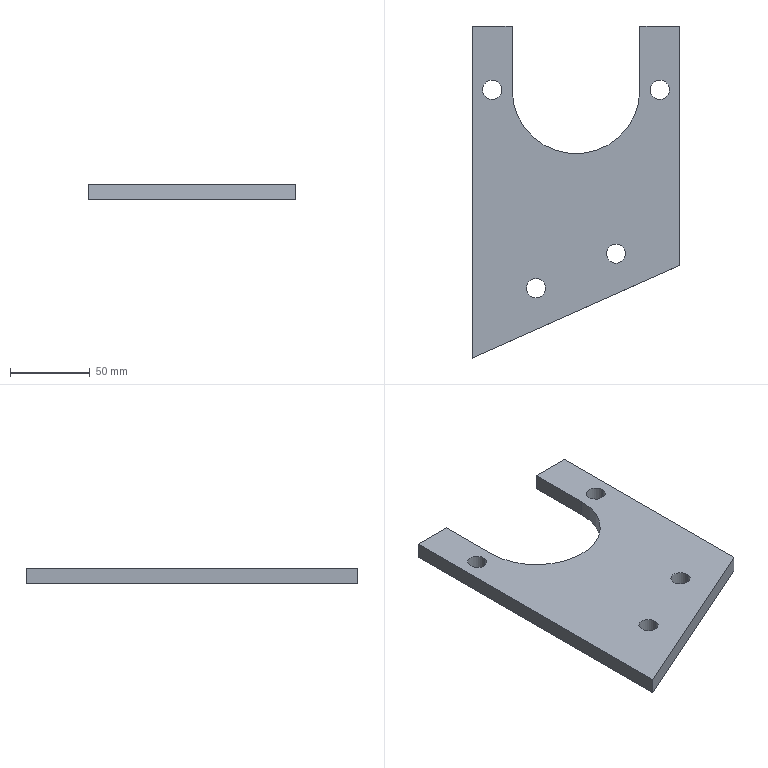Part | SolidWorks | features Extrusion 1 | 1 solid | 18 faces | box 130 x 208 x 10 mm | volume 171043 mm3 | cylinder 9 | plane 9 | commonest cylinder face diameters 12 x8 80 x1
STEP:
#1=CARTESIAN_POINT('',(84.,65.43,10.));
#2=VERTEX_POINT('',#1);
#3=CARTESIAN_POINT('',(96.,65.43,10.));
#4=VERTEX_POINT('',#3);
#5=CARTESIAN_POINT('',(90.,65.43,10.));
#6=DIRECTION('',(0.,0.,1.));
#7=DIRECTION('',(1.,0.,0.));
#8=AXIS2_PLACEMENT_3D('',#5,#6,#7);
#9=CIRCLE('',#8,6.);
#10=EDGE_CURVE('',#2,#4,#9,.T.);
#11=ORIENTED_EDGE('',*,*,#10,.T.);
#12=CARTESIAN_POINT('',(96.,65.43,0.));
#13=VERTEX_POINT('',#12);
#14=CARTESIAN_POINT('',(96.,65.43,10.));
#15=DIRECTION('',(0.,0.,-1.));
#16=VECTOR('',#15,1000.);
#17=LINE('',#14,#16);
#18=EDGE_CURVE('',#4,#13,#17,.T.);
#19=ORIENTED_EDGE('',*,*,#18,.T.);
#20=CARTESIAN_POINT('',(84.,65.43,0.));
#21=VERTEX_POINT('',#20);
#22=CARTESIAN_POINT('',(90.,65.43,0.));
#23=DIRECTION('',(0.,0.,1.));
#24=DIRECTION('',(1.,0.,0.));
#25=AXIS2_PLACEMENT_3D('',#22,#23,#24);
#26=CIRCLE('',#25,6.);
#27=EDGE_CURVE('',#21,#13,#26,.T.);
#28=ORIENTED_EDGE('',*,*,#27,.F.);
#29=CARTESIAN_POINT('',(84.,65.43,10.));
#30=DIRECTION('',(0.,0.,-1.));
#31=VECTOR('',#30,1000.);
#32=LINE('',#29,#31);
#33=EDGE_CURVE('',#2,#21,#32,.T.);
#34=ORIENTED_EDGE('',*,*,#33,.F.);
#35=EDGE_LOOP('',(#11,#19,#28,#34));
#36=FACE_OUTER_BOUND('',#35,.T.);
#37=CARTESIAN_POINT('',(90.,65.43,10.));
#38=DIRECTION('',(0.,0.,-1.));
#39=DIRECTION('',(-1.,0.,0.));
#40=AXIS2_PLACEMENT_3D('',#37,#38,#39);
#41=CYLINDRICAL_SURFACE('',#40,6.);
#42=ADVANCED_FACE('',(#36),#41,.F.);
#43=CARTESIAN_POINT('',(34.,43.72,10.));
#44=VERTEX_POINT('',#43);
#45=CARTESIAN_POINT('',(46.,43.72,10.));
#46=VERTEX_POINT('',#45);
#47=CARTESIAN_POINT('',(40.,43.72,10.));
#48=DIRECTION('',(0.,0.,1.));
#49=DIRECTION('',(1.,0.,0.));
#50=AXIS2_PLACEMENT_3D('',#47,#48,#49);
#51=CIRCLE('',#50,6.);
#52=EDGE_CURVE('',#44,#46,#51,.T.);
#53=ORIENTED_EDGE('',*,*,#52,.T.);
#54=CARTESIAN_POINT('',(46.,43.72,0.));
#55=VERTEX_POINT('',#54);
#56=CARTESIAN_POINT('',(46.,43.72,10.));
#57=DIRECTION('',(0.,0.,-1.));
#58=VECTOR('',#57,1000.);
#59=LINE('',#56,#58);
#60=EDGE_CURVE('',#46,#55,#59,.T.);
#61=ORIENTED_EDGE('',*,*,#60,.T.);
#62=CARTESIAN_POINT('',(34.,43.72,0.));
#63=VERTEX_POINT('',#62);
#64=CARTESIAN_POINT('',(40.,43.72,0.));
#65=DIRECTION('',(0.,0.,1.));
#66=DIRECTION('',(1.,0.,0.));
#67=AXIS2_PLACEMENT_3D('',#64,#65,#66);
#68=CIRCLE('',#67,6.);
#69=EDGE_CURVE('',#63,#55,#68,.T.);
#70=ORIENTED_EDGE('',*,*,#69,.F.);
#71=CARTESIAN_POINT('',(34.,43.72,10.));
#72=DIRECTION('',(0.,0.,-1.));
#73=VECTOR('',#72,1000.);
#74=LINE('',#71,#73);
#75=EDGE_CURVE('',#44,#63,#74,.T.);
#76=ORIENTED_EDGE('',*,*,#75,.F.);
#77=EDGE_LOOP('',(#53,#61,#70,#76));
#78=FACE_OUTER_BOUND('',#77,.T.);
#79=CARTESIAN_POINT('',(40.,43.72,10.));
#80=DIRECTION('',(0.,0.,-1.));
#81=DIRECTION('',(-1.,0.,0.));
#82=AXIS2_PLACEMENT_3D('',#79,#80,#81);
#83=CYLINDRICAL_SURFACE('',#82,6.);
#84=ADVANCED_FACE('',(#78),#83,.F.);
#85=CARTESIAN_POINT('',(6.5,168.,10.));
#86=VERTEX_POINT('',#85);
#87=CARTESIAN_POINT('',(18.5,168.,10.));
#88=VERTEX_POINT('',#87);
#89=CARTESIAN_POINT('',(12.5,168.,10.));
#90=DIRECTION('',(0.,0.,1.));
#91=DIRECTION('',(1.,0.,0.));
#92=AXIS2_PLACEMENT_3D('',#89,#90,#91);
#93=CIRCLE('',#92,6.);
#94=EDGE_CURVE('',#86,#88,#93,.T.);
#95=ORIENTED_EDGE('',*,*,#94,.T.);
#96=CARTESIAN_POINT('',(18.5,168.,0.));
#97=VERTEX_POINT('',#96);
#98=CARTESIAN_POINT('',(18.5,168.,10.));
#99=DIRECTION('',(0.,0.,-1.));
#100=VECTOR('',#99,1000.);
#101=LINE('',#98,#100);
#102=EDGE_CURVE('',#88,#97,#101,.T.);
#103=ORIENTED_EDGE('',*,*,#102,.T.);
#104=CARTESIAN_POINT('',(6.5,168.,0.));
#105=VERTEX_POINT('',#104);
#106=CARTESIAN_POINT('',(12.5,168.,0.));
#107=DIRECTION('',(0.,0.,1.));
#108=DIRECTION('',(1.,0.,0.));
#109=AXIS2_PLACEMENT_3D('',#106,#107,#108);
#110=CIRCLE('',#109,6.);
#111=EDGE_CURVE('',#105,#97,#110,.T.);
#112=ORIENTED_EDGE('',*,*,#111,.F.);
#113=CARTESIAN_POINT('',(6.5,168.,10.));
#114=DIRECTION('',(0.,0.,-1.));
#115=VECTOR('',#114,1000.);
#116=LINE('',#113,#115);
#117=EDGE_CURVE('',#86,#105,#116,.T.);
#118=ORIENTED_EDGE('',*,*,#117,.F.);
#119=EDGE_LOOP('',(#95,#103,#112,#118));
#120=FACE_OUTER_BOUND('',#119,.T.);
#121=CARTESIAN_POINT('',(12.5,168.,10.));
#122=DIRECTION('',(0.,0.,-1.));
#123=DIRECTION('',(-1.,0.,0.));
#124=AXIS2_PLACEMENT_3D('',#121,#122,#123);
#125=CYLINDRICAL_SURFACE('',#124,6.);
#126=ADVANCED_FACE('',(#120),#125,.F.);
#127=CARTESIAN_POINT('',(111.5,168.,10.));
#128=VERTEX_POINT('',#127);
#129=CARTESIAN_POINT('',(123.5,168.,10.));
#130=VERTEX_POINT('',#129);
#131=CARTESIAN_POINT('',(117.5,168.,10.));
#132=DIRECTION('',(0.,0.,1.));
#133=DIRECTION('',(1.,0.,0.));
#134=AXIS2_PLACEMENT_3D('',#131,#132,#133);
#135=CIRCLE('',#134,6.);
#136=EDGE_CURVE('',#128,#130,#135,.T.);
#137=ORIENTED_EDGE('',*,*,#136,.T.);
#138=CARTESIAN_POINT('',(123.5,168.,0.));
#139=VERTEX_POINT('',#138);
#140=CARTESIAN_POINT('',(123.5,168.,10.));
#141=DIRECTION('',(0.,0.,-1.));
#142=VECTOR('',#141,1000.);
#143=LINE('',#140,#142);
#144=EDGE_CURVE('',#130,#139,#143,.T.);
#145=ORIENTED_EDGE('',*,*,#144,.T.);
#146=CARTESIAN_POINT('',(111.5,168.,0.));
#147=VERTEX_POINT('',#146);
#148=CARTESIAN_POINT('',(117.5,168.,0.));
#149=DIRECTION('',(0.,0.,1.));
#150=DIRECTION('',(1.,0.,0.));
#151=AXIS2_PLACEMENT_3D('',#148,#149,#150);
#152=CIRCLE('',#151,6.);
#153=EDGE_CURVE('',#147,#139,#152,.T.);
#154=ORIENTED_EDGE('',*,*,#153,.F.);
#155=CARTESIAN_POINT('',(111.5,168.,10.));
#156=DIRECTION('',(0.,0.,-1.));
#157=VECTOR('',#156,1000.);
#158=LINE('',#155,#157);
#159=EDGE_CURVE('',#128,#147,#158,.T.);
#160=ORIENTED_EDGE('',*,*,#159,.F.);
#161=EDGE_LOOP('',(#137,#145,#154,#160));
#162=FACE_OUTER_BOUND('',#161,.T.);
#163=CARTESIAN_POINT('',(117.5,168.,10.));
#164=DIRECTION('',(0.,0.,-1.));
#165=DIRECTION('',(-1.,0.,0.));
#166=AXIS2_PLACEMENT_3D('',#163,#164,#165);
#167=CYLINDRICAL_SURFACE('',#166,6.);
#168=ADVANCED_FACE('',(#162),#167,.F.);
#169=ORIENTED_EDGE('',*,*,#52,.F.);
#170=CARTESIAN_POINT('',(40.,43.72,10.));
#171=DIRECTION('',(0.,0.,1.));
#172=DIRECTION('',(1.,0.,0.));
#173=AXIS2_PLACEMENT_3D('',#170,#171,#172);
#174=CIRCLE('',#173,6.);
#175=EDGE_CURVE('',#46,#44,#174,.T.);
#176=ORIENTED_EDGE('',*,*,#175,.F.);
#177=EDGE_LOOP('',(#169,#176));
#178=FACE_BOUND('',#177,.T.);
#179=ORIENTED_EDGE('',*,*,#136,.F.);
#180=CARTESIAN_POINT('',(117.5,168.,10.));
#181=DIRECTION('',(0.,0.,1.));
#182=DIRECTION('',(1.,0.,0.));
#183=AXIS2_PLACEMENT_3D('',#180,#181,#182);
#184=CIRCLE('',#183,6.);
#185=EDGE_CURVE('',#130,#128,#184,.T.);
#186=ORIENTED_EDGE('',*,*,#185,.F.);
#187=EDGE_LOOP('',(#179,#186));
#188=FACE_BOUND('',#187,.T.);
#189=CARTESIAN_POINT('',(0.,0.,10.));
#190=VERTEX_POINT('',#189);
#191=CARTESIAN_POINT('',(130.,58.,10.));
#192=VERTEX_POINT('',#191);
#193=CARTESIAN_POINT('',(130.,58.,10.));
#194=DIRECTION('',(0.9132,0.4074,0.));
#195=VECTOR('',#194,1000.);
#196=LINE('',#193,#195);
#197=EDGE_CURVE('',#190,#192,#196,.T.);
#198=ORIENTED_EDGE('',*,*,#197,.T.);
#199=CARTESIAN_POINT('',(130.,208.,10.));
#200=VERTEX_POINT('',#199);
#201=CARTESIAN_POINT('',(130.,208.,10.));
#202=DIRECTION('',(0.,1.,0.));
#203=VECTOR('',#202,1000.);
#204=LINE('',#201,#203);
#205=EDGE_CURVE('',#192,#200,#204,.T.);
#206=ORIENTED_EDGE('',*,*,#205,.T.);
#207=CARTESIAN_POINT('',(105.,208.,10.));
#208=VERTEX_POINT('',#207);
#209=CARTESIAN_POINT('',(105.,208.,10.));
#210=DIRECTION('',(-1.,0.,0.));
#211=VECTOR('',#210,1000.);
#212=LINE('',#209,#211);
#213=EDGE_CURVE('',#200,#208,#212,.T.);
#214=ORIENTED_EDGE('',*,*,#213,.T.);
#215=CARTESIAN_POINT('',(105.,168.,10.));
#216=VERTEX_POINT('',#215);
#217=CARTESIAN_POINT('',(105.,168.,10.));
#218=DIRECTION('',(0.,-1.,0.));
#219=VECTOR('',#218,1000.);
#220=LINE('',#217,#219);
#221=EDGE_CURVE('',#208,#216,#220,.T.);
#222=ORIENTED_EDGE('',*,*,#221,.T.);
#223=CARTESIAN_POINT('',(25.,168.,10.));
#224=VERTEX_POINT('',#223);
#225=CARTESIAN_POINT('',(65.,168.,10.));
#226=DIRECTION('',(0.,0.,-1.));
#227=DIRECTION('',(1.,0.,0.));
#228=AXIS2_PLACEMENT_3D('',#225,#226,#227);
#229=CIRCLE('',#228,40.);
#230=EDGE_CURVE('',#216,#224,#229,.T.);
#231=ORIENTED_EDGE('',*,*,#230,.T.);
#232=CARTESIAN_POINT('',(25.,208.,10.));
#233=VERTEX_POINT('',#232);
#234=CARTESIAN_POINT('',(25.,168.,10.));
#235=DIRECTION('',(0.,1.,0.));
#236=VECTOR('',#235,1000.);
#237=LINE('',#234,#236);
#238=EDGE_CURVE('',#224,#233,#237,.T.);
#239=ORIENTED_EDGE('',*,*,#238,.T.);
#240=CARTESIAN_POINT('',(0.,208.,10.));
#241=VERTEX_POINT('',#240);
#242=CARTESIAN_POINT('',(0.,208.,10.));
#243=DIRECTION('',(-1.,0.,0.));
#244=VECTOR('',#243,1000.);
#245=LINE('',#242,#244);
#246=EDGE_CURVE('',#233,#241,#245,.T.);
#247=ORIENTED_EDGE('',*,*,#246,.T.);
#248=CARTESIAN_POINT('',(0.,0.,10.));
#249=DIRECTION('',(0.,-1.,0.));
#250=VECTOR('',#249,1000.);
#251=LINE('',#248,#250);
#252=EDGE_CURVE('',#241,#190,#251,.T.);
#253=ORIENTED_EDGE('',*,*,#252,.T.);
#254=EDGE_LOOP('',(#198,#206,#214,#222,#231,#239,#247,#253));
#255=FACE_OUTER_BOUND('',#254,.T.);
#256=ORIENTED_EDGE('',*,*,#94,.F.);
#257=CARTESIAN_POINT('',(12.5,168.,10.));
#258=DIRECTION('',(0.,0.,1.));
#259=DIRECTION('',(1.,0.,0.));
#260=AXIS2_PLACEMENT_3D('',#257,#258,#259);
#261=CIRCLE('',#260,6.);
#262=EDGE_CURVE('',#88,#86,#261,.T.);
#263=ORIENTED_EDGE('',*,*,#262,.F.);
#264=EDGE_LOOP('',(#256,#263));
#265=FACE_BOUND('',#264,.T.);
#266=ORIENTED_EDGE('',*,*,#10,.F.);
#267=CARTESIAN_POINT('',(90.,65.43,10.));
#268=DIRECTION('',(0.,0.,1.));
#269=DIRECTION('',(1.,0.,0.));
#270=AXIS2_PLACEMENT_3D('',#267,#268,#269);
#271=CIRCLE('',#270,6.);
#272=EDGE_CURVE('',#4,#2,#271,.T.);
#273=ORIENTED_EDGE('',*,*,#272,.F.);
#274=EDGE_LOOP('',(#266,#273));
#275=FACE_BOUND('',#274,.T.);
#276=CARTESIAN_POINT('',(65.,168.,10.));
#277=DIRECTION('',(0.,0.,1.));
#278=DIRECTION('',(1.,0.,0.));
#279=AXIS2_PLACEMENT_3D('',#276,#277,#278);
#280=PLANE('',#279);
#281=ADVANCED_FACE('',(#178,#188,#255,#265,#275),#280,.T.);
#282=ORIENTED_EDGE('',*,*,#69,.T.);
#283=CARTESIAN_POINT('',(40.,43.72,0.));
#284=DIRECTION('',(0.,0.,1.));
#285=DIRECTION('',(1.,0.,0.));
#286=AXIS2_PLACEMENT_3D('',#283,#284,#285);
#287=CIRCLE('',#286,6.);
#288=EDGE_CURVE('',#55,#63,#287,.T.);
#289=ORIENTED_EDGE('',*,*,#288,.T.);
#290=EDGE_LOOP('',(#282,#289));
#291=FACE_BOUND('',#290,.T.);
#292=ORIENTED_EDGE('',*,*,#153,.T.);
#293=CARTESIAN_POINT('',(117.5,168.,0.));
#294=DIRECTION('',(0.,0.,1.));
#295=DIRECTION('',(1.,0.,0.));
#296=AXIS2_PLACEMENT_3D('',#293,#294,#295);
#297=CIRCLE('',#296,6.);
#298=EDGE_CURVE('',#139,#147,#297,.T.);
#299=ORIENTED_EDGE('',*,*,#298,.T.);
#300=EDGE_LOOP('',(#292,#299));
#301=FACE_BOUND('',#300,.T.);
#302=CARTESIAN_POINT('',(0.,0.,0.));
#303=VERTEX_POINT('',#302);
#304=CARTESIAN_POINT('',(130.,58.,0.));
#305=VERTEX_POINT('',#304);
#306=CARTESIAN_POINT('',(130.,58.,0.));
#307=DIRECTION('',(0.9132,0.4074,0.));
#308=VECTOR('',#307,1000.);
#309=LINE('',#306,#308);
#310=EDGE_CURVE('',#303,#305,#309,.T.);
#311=ORIENTED_EDGE('',*,*,#310,.F.);
#312=CARTESIAN_POINT('',(0.,208.,0.));
#313=VERTEX_POINT('',#312);
#314=CARTESIAN_POINT('',(0.,0.,0.));
#315=DIRECTION('',(0.,-1.,0.));
#316=VECTOR('',#315,1000.);
#317=LINE('',#314,#316);
#318=EDGE_CURVE('',#313,#303,#317,.T.);
#319=ORIENTED_EDGE('',*,*,#318,.F.);
#320=CARTESIAN_POINT('',(25.,208.,0.));
#321=VERTEX_POINT('',#320);
#322=CARTESIAN_POINT('',(0.,208.,0.));
#323=DIRECTION('',(-1.,0.,0.));
#324=VECTOR('',#323,1000.);
#325=LINE('',#322,#324);
#326=EDGE_CURVE('',#321,#313,#325,.T.);
#327=ORIENTED_EDGE('',*,*,#326,.F.);
#328=CARTESIAN_POINT('',(25.,168.,0.));
#329=VERTEX_POINT('',#328);
#330=CARTESIAN_POINT('',(25.,168.,0.));
#331=DIRECTION('',(0.,1.,0.));
#332=VECTOR('',#331,1000.);
#333=LINE('',#330,#332);
#334=EDGE_CURVE('',#329,#321,#333,.T.);
#335=ORIENTED_EDGE('',*,*,#334,.F.);
#336=CARTESIAN_POINT('',(105.,168.,0.));
#337=VERTEX_POINT('',#336);
#338=CARTESIAN_POINT('',(65.,168.,0.));
#339=DIRECTION('',(0.,0.,-1.));
#340=DIRECTION('',(1.,0.,0.));
#341=AXIS2_PLACEMENT_3D('',#338,#339,#340);
#342=CIRCLE('',#341,40.);
#343=EDGE_CURVE('',#337,#329,#342,.T.);
#344=ORIENTED_EDGE('',*,*,#343,.F.);
#345=CARTESIAN_POINT('',(105.,208.,0.));
#346=VERTEX_POINT('',#345);
#347=CARTESIAN_POINT('',(105.,168.,0.));
#348=DIRECTION('',(0.,-1.,0.));
#349=VECTOR('',#348,1000.);
#350=LINE('',#347,#349);
#351=EDGE_CURVE('',#346,#337,#350,.T.);
#352=ORIENTED_EDGE('',*,*,#351,.F.);
#353=CARTESIAN_POINT('',(130.,208.,0.));
#354=VERTEX_POINT('',#353);
#355=CARTESIAN_POINT('',(105.,208.,0.));
#356=DIRECTION('',(-1.,0.,0.));
#357=VECTOR('',#356,1000.);
#358=LINE('',#355,#357);
#359=EDGE_CURVE('',#354,#346,#358,.T.);
#360=ORIENTED_EDGE('',*,*,#359,.F.);
#361=CARTESIAN_POINT('',(130.,208.,0.));
#362=DIRECTION('',(0.,1.,0.));
#363=VECTOR('',#362,1000.);
#364=LINE('',#361,#363);
#365=EDGE_CURVE('',#305,#354,#364,.T.);
#366=ORIENTED_EDGE('',*,*,#365,.F.);
#367=EDGE_LOOP('',(#311,#319,#327,#335,#344,#352,#360,#366));
#368=FACE_OUTER_BOUND('',#367,.T.);
#369=ORIENTED_EDGE('',*,*,#111,.T.);
#370=CARTESIAN_POINT('',(12.5,168.,0.));
#371=DIRECTION('',(0.,0.,1.));
#372=DIRECTION('',(1.,0.,0.));
#373=AXIS2_PLACEMENT_3D('',#370,#371,#372);
#374=CIRCLE('',#373,6.);
#375=EDGE_CURVE('',#97,#105,#374,.T.);
#376=ORIENTED_EDGE('',*,*,#375,.T.);
#377=EDGE_LOOP('',(#369,#376));
#378=FACE_BOUND('',#377,.T.);
#379=ORIENTED_EDGE('',*,*,#27,.T.);
#380=CARTESIAN_POINT('',(90.,65.43,0.));
#381=DIRECTION('',(0.,0.,1.));
#382=DIRECTION('',(1.,0.,0.));
#383=AXIS2_PLACEMENT_3D('',#380,#381,#382);
#384=CIRCLE('',#383,6.);
#385=EDGE_CURVE('',#13,#21,#384,.T.);
#386=ORIENTED_EDGE('',*,*,#385,.T.);
#387=EDGE_LOOP('',(#379,#386));
#388=FACE_BOUND('',#387,.T.);
#389=CARTESIAN_POINT('',(65.,168.,0.));
#390=DIRECTION('',(0.,0.,1.));
#391=DIRECTION('',(1.,0.,0.));
#392=AXIS2_PLACEMENT_3D('',#389,#390,#391);
#393=PLANE('',#392);
#394=ADVANCED_FACE('',(#291,#301,#368,#378,#388),#393,.F.);
#395=ORIENTED_EDGE('',*,*,#310,.T.);
#396=CARTESIAN_POINT('',(130.,58.,10.));
#397=DIRECTION('',(0.,0.,-1.));
#398=VECTOR('',#397,1000.);
#399=LINE('',#396,#398);
#400=EDGE_CURVE('',#192,#305,#399,.T.);
#401=ORIENTED_EDGE('',*,*,#400,.F.);
#402=ORIENTED_EDGE('',*,*,#197,.F.);
#403=CARTESIAN_POINT('',(0.,0.,10.));
#404=DIRECTION('',(0.,0.,-1.));
#405=VECTOR('',#404,1000.);
#406=LINE('',#403,#405);
#407=EDGE_CURVE('',#190,#303,#406,.T.);
#408=ORIENTED_EDGE('',*,*,#407,.T.);
#409=EDGE_LOOP('',(#395,#401,#402,#408));
#410=FACE_OUTER_BOUND('',#409,.T.);
#411=CARTESIAN_POINT('',(130.,58.,10.));
#412=DIRECTION('',(-0.4074,0.9132,0.));
#413=DIRECTION('',(-0.9132,-0.4074,0.));
#414=AXIS2_PLACEMENT_3D('',#411,#412,#413);
#415=PLANE('',#414);
#416=ADVANCED_FACE('',(#410),#415,.F.);
#417=ORIENTED_EDGE('',*,*,#365,.T.);
#418=CARTESIAN_POINT('',(130.,208.,10.));
#419=DIRECTION('',(0.,0.,-1.));
#420=VECTOR('',#419,1000.);
#421=LINE('',#418,#420);
#422=EDGE_CURVE('',#200,#354,#421,.T.);
#423=ORIENTED_EDGE('',*,*,#422,.F.);
#424=ORIENTED_EDGE('',*,*,#205,.F.);
#425=ORIENTED_EDGE('',*,*,#400,.T.);
#426=EDGE_LOOP('',(#417,#423,#424,#425));
#427=FACE_OUTER_BOUND('',#426,.T.);
#428=CARTESIAN_POINT('',(130.,208.,10.));
#429=DIRECTION('',(-1.,0.,0.));
#430=DIRECTION('',(0.,0.,1.));
#431=AXIS2_PLACEMENT_3D('',#428,#429,#430);
#432=PLANE('',#431);
#433=ADVANCED_FACE('',(#427),#432,.F.);
#434=ORIENTED_EDGE('',*,*,#359,.T.);
#435=CARTESIAN_POINT('',(105.,208.,10.));
#436=DIRECTION('',(0.,0.,-1.));
#437=VECTOR('',#436,1000.);
#438=LINE('',#435,#437);
#439=EDGE_CURVE('',#208,#346,#438,.T.);
#440=ORIENTED_EDGE('',*,*,#439,.F.);
#441=ORIENTED_EDGE('',*,*,#213,.F.);
#442=ORIENTED_EDGE('',*,*,#422,.T.);
#443=EDGE_LOOP('',(#434,#440,#441,#442));
#444=FACE_OUTER_BOUND('',#443,.T.);
#445=CARTESIAN_POINT('',(105.,208.,10.));
#446=DIRECTION('',(0.,-1.,0.));
#447=DIRECTION('',(0.,0.,-1.));
#448=AXIS2_PLACEMENT_3D('',#445,#446,#447);
#449=PLANE('',#448);
#450=ADVANCED_FACE('',(#444),#449,.F.);
#451=ORIENTED_EDGE('',*,*,#351,.T.);
#452=CARTESIAN_POINT('',(105.,168.,10.));
#453=DIRECTION('',(0.,0.,-1.));
#454=VECTOR('',#453,1000.);
#455=LINE('',#452,#454);
#456=EDGE_CURVE('',#216,#337,#455,.T.);
#457=ORIENTED_EDGE('',*,*,#456,.F.);
#458=ORIENTED_EDGE('',*,*,#221,.F.);
#459=ORIENTED_EDGE('',*,*,#439,.T.);
#460=EDGE_LOOP('',(#451,#457,#458,#459));
#461=FACE_OUTER_BOUND('',#460,.T.);
#462=CARTESIAN_POINT('',(105.,168.,10.));
#463=DIRECTION('',(1.,0.,0.));
#464=DIRECTION('',(0.,0.,-1.));
#465=AXIS2_PLACEMENT_3D('',#462,#463,#464);
#466=PLANE('',#465);
#467=ADVANCED_FACE('',(#461),#466,.F.);
#468=ORIENTED_EDGE('',*,*,#343,.T.);
#469=CARTESIAN_POINT('',(25.,168.,10.));
#470=DIRECTION('',(0.,0.,-1.));
#471=VECTOR('',#470,1000.);
#472=LINE('',#469,#471);
#473=EDGE_CURVE('',#224,#329,#472,.T.);
#474=ORIENTED_EDGE('',*,*,#473,.F.);
#475=ORIENTED_EDGE('',*,*,#230,.F.);
#476=ORIENTED_EDGE('',*,*,#456,.T.);
#477=EDGE_LOOP('',(#468,#474,#475,#476));
#478=FACE_OUTER_BOUND('',#477,.T.);
#479=CARTESIAN_POINT('',(65.,168.,10.));
#480=DIRECTION('',(0.,0.,-1.));
#481=DIRECTION('',(-1.,0.,0.));
#482=AXIS2_PLACEMENT_3D('',#479,#480,#481);
#483=CYLINDRICAL_SURFACE('',#482,40.);
#484=ADVANCED_FACE('',(#478),#483,.F.);
#485=ORIENTED_EDGE('',*,*,#334,.T.);
#486=CARTESIAN_POINT('',(25.,208.,10.));
#487=DIRECTION('',(0.,0.,-1.));
#488=VECTOR('',#487,1000.);
#489=LINE('',#486,#488);
#490=EDGE_CURVE('',#233,#321,#489,.T.);
#491=ORIENTED_EDGE('',*,*,#490,.F.);
#492=ORIENTED_EDGE('',*,*,#238,.F.);
#493=ORIENTED_EDGE('',*,*,#473,.T.);
#494=EDGE_LOOP('',(#485,#491,#492,#493));
#495=FACE_OUTER_BOUND('',#494,.T.);
#496=CARTESIAN_POINT('',(25.,168.,10.));
#497=DIRECTION('',(-1.,0.,0.));
#498=DIRECTION('',(0.,0.,1.));
#499=AXIS2_PLACEMENT_3D('',#496,#497,#498);
#500=PLANE('',#499);
#501=ADVANCED_FACE('',(#495),#500,.F.);
#502=ORIENTED_EDGE('',*,*,#326,.T.);
#503=CARTESIAN_POINT('',(0.,208.,10.));
#504=DIRECTION('',(0.,0.,-1.));
#505=VECTOR('',#504,1000.);
#506=LINE('',#503,#505);
#507=EDGE_CURVE('',#241,#313,#506,.T.);
#508=ORIENTED_EDGE('',*,*,#507,.F.);
#509=ORIENTED_EDGE('',*,*,#246,.F.);
#510=ORIENTED_EDGE('',*,*,#490,.T.);
#511=EDGE_LOOP('',(#502,#508,#509,#510));
#512=FACE_OUTER_BOUND('',#511,.T.);
#513=CARTESIAN_POINT('',(0.,208.,10.));
#514=DIRECTION('',(0.,-1.,0.));
#515=DIRECTION('',(0.,0.,-1.));
#516=AXIS2_PLACEMENT_3D('',#513,#514,#515);
#517=PLANE('',#516);
#518=ADVANCED_FACE('',(#512),#517,.F.);
#519=ORIENTED_EDGE('',*,*,#318,.T.);
#520=ORIENTED_EDGE('',*,*,#407,.F.);
#521=ORIENTED_EDGE('',*,*,#252,.F.);
#522=ORIENTED_EDGE('',*,*,#507,.T.);
#523=EDGE_LOOP('',(#519,#520,#521,#522));
#524=FACE_OUTER_BOUND('',#523,.T.);
#525=CARTESIAN_POINT('',(0.,0.,10.));
#526=DIRECTION('',(1.,0.,0.));
#527=DIRECTION('',(0.,0.,-1.));
#528=AXIS2_PLACEMENT_3D('',#525,#526,#527);
#529=PLANE('',#528);
#530=ADVANCED_FACE('',(#524),#529,.F.);
#531=ORIENTED_EDGE('',*,*,#144,.F.);
#532=ORIENTED_EDGE('',*,*,#185,.T.);
#533=ORIENTED_EDGE('',*,*,#159,.T.);
#534=ORIENTED_EDGE('',*,*,#298,.F.);
#535=EDGE_LOOP('',(#531,#532,#533,#534));
#536=FACE_OUTER_BOUND('',#535,.T.);
#537=CARTESIAN_POINT('',(117.5,168.,10.));
#538=DIRECTION('',(0.,0.,-1.));
#539=DIRECTION('',(-1.,0.,0.));
#540=AXIS2_PLACEMENT_3D('',#537,#538,#539);
#541=CYLINDRICAL_SURFACE('',#540,6.);
#542=ADVANCED_FACE('',(#536),#541,.F.);
#543=ORIENTED_EDGE('',*,*,#102,.F.);
#544=ORIENTED_EDGE('',*,*,#262,.T.);
#545=ORIENTED_EDGE('',*,*,#117,.T.);
#546=ORIENTED_EDGE('',*,*,#375,.F.);
#547=EDGE_LOOP('',(#543,#544,#545,#546));
#548=FACE_OUTER_BOUND('',#547,.T.);
#549=CARTESIAN_POINT('',(12.5,168.,10.));
#550=DIRECTION('',(0.,0.,-1.));
#551=DIRECTION('',(-1.,0.,0.));
#552=AXIS2_PLACEMENT_3D('',#549,#550,#551);
#553=CYLINDRICAL_SURFACE('',#552,6.);
#554=ADVANCED_FACE('',(#548),#553,.F.);
#555=ORIENTED_EDGE('',*,*,#60,.F.);
#556=ORIENTED_EDGE('',*,*,#175,.T.);
#557=ORIENTED_EDGE('',*,*,#75,.T.);
#558=ORIENTED_EDGE('',*,*,#288,.F.);
#559=EDGE_LOOP('',(#555,#556,#557,#558));
#560=FACE_OUTER_BOUND('',#559,.T.);
#561=CARTESIAN_POINT('',(40.,43.72,10.));
#562=DIRECTION('',(0.,0.,-1.));
#563=DIRECTION('',(-1.,0.,0.));
#564=AXIS2_PLACEMENT_3D('',#561,#562,#563);
#565=CYLINDRICAL_SURFACE('',#564,6.);
#566=ADVANCED_FACE('',(#560),#565,.F.);
#567=ORIENTED_EDGE('',*,*,#18,.F.);
#568=ORIENTED_EDGE('',*,*,#272,.T.);
#569=ORIENTED_EDGE('',*,*,#33,.T.);
#570=ORIENTED_EDGE('',*,*,#385,.F.);
#571=EDGE_LOOP('',(#567,#568,#569,#570));
#572=FACE_OUTER_BOUND('',#571,.T.);
#573=CARTESIAN_POINT('',(90.,65.43,10.));
#574=DIRECTION('',(0.,0.,-1.));
#575=DIRECTION('',(-1.,0.,0.));
#576=AXIS2_PLACEMENT_3D('',#573,#574,#575);
#577=CYLINDRICAL_SURFACE('',#576,6.);
#578=ADVANCED_FACE('',(#572),#577,.F.);
#579=CLOSED_SHELL('',(#42,#84,#126,#168,#281,#394,#416,#433,#450,#467,#484,#501,#518,#530,#542,#554,#566,#578));
#580=MANIFOLD_SOLID_BREP('',#579);
#581=CARTESIAN_POINT('',(0.,0.,0.));
#582=DIRECTION('',(0.,0.,1.));
#583=DIRECTION('',(1.,0.,0.));
#584=AXIS2_PLACEMENT_3D('',#581,#582,#583);
#585=(LENGTH_UNIT()NAMED_UNIT(*)SI_UNIT(.MILLI.,.METRE.));
#586=UNCERTAINTY_MEASURE_WITH_UNIT(LENGTH_MEASURE(0.00001),#585,'','');
#587=(NAMED_UNIT(*)PLANE_ANGLE_UNIT()SI_UNIT($,.RADIAN.));
#588=(NAMED_UNIT(*)SI_UNIT($,.STERADIAN.)SOLID_ANGLE_UNIT());
#589=(GEOMETRIC_REPRESENTATION_CONTEXT(3)GLOBAL_UNCERTAINTY_ASSIGNED_CONTEXT((#586))GLOBAL_UNIT_ASSIGNED_CONTEXT((#585,#587,#588))REPRESENTATION_CONTEXT('',''));
#590=ADVANCED_BREP_SHAPE_REPRESENTATION('',(#580,#584),#589);